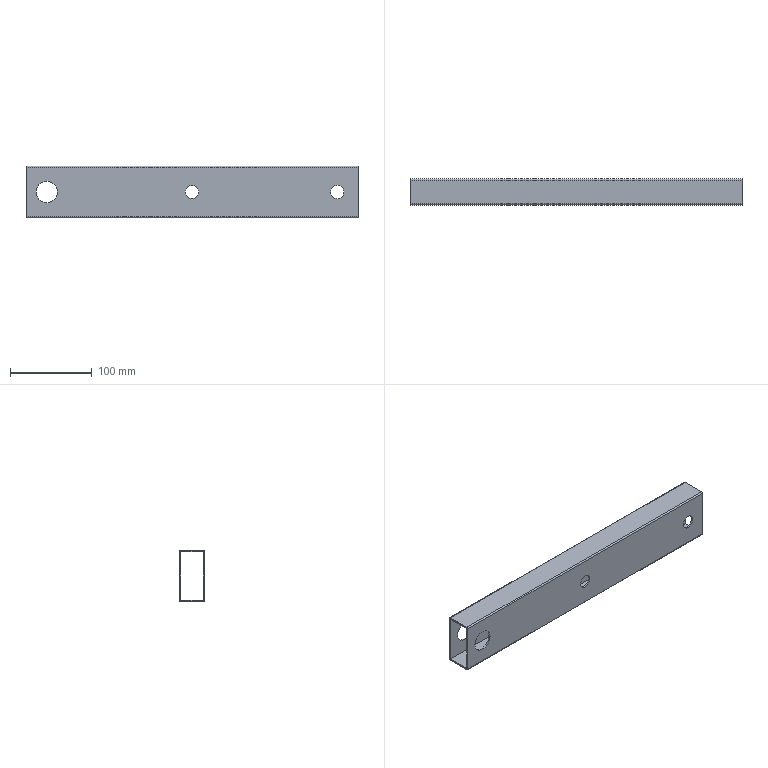Part | NX | features BREP 1 | 1 solid | 26 faces | box 406.4 x 31.75 x 63.5 mm | volume 142348 mm3 | cylinder 16 | plane 10 | commonest cylinder face diameters 16.256 x8 3.175 x4 26.162 x4
STEP:
#1=CARTESIAN_POINT('',(-203.2,15.875,-30.163));
#2=VERTEX_POINT('',#1);
#3=CARTESIAN_POINT('',(-203.2,15.875,30.163));
#4=VERTEX_POINT('',#3);
#5=CARTESIAN_POINT('',(-203.2,15.875,-30.163));
#6=DIRECTION('',(0.,0.,1.));
#7=VECTOR('',#6,1000.);
#8=LINE('',#5,#7);
#9=EDGE_CURVE('',#2,#4,#8,.T.);
#10=ORIENTED_EDGE('',*,*,#9,.F.);
#11=CARTESIAN_POINT('',(-203.2,14.287,-31.75));
#12=VERTEX_POINT('',#11);
#13=CARTESIAN_POINT('',(-203.2,14.287,-30.163));
#14=DIRECTION('',(-1.,0.,0.));
#15=DIRECTION('',(0.,1.,0.));
#16=AXIS2_PLACEMENT_3D('',#13,#14,#15);
#17=CIRCLE('',#16,1.587);
#18=EDGE_CURVE('',#2,#12,#17,.T.);
#19=ORIENTED_EDGE('',*,*,#18,.T.);
#20=CARTESIAN_POINT('',(-203.2,-14.287,-31.75));
#21=VERTEX_POINT('',#20);
#22=CARTESIAN_POINT('',(-203.2,-14.287,-31.75));
#23=DIRECTION('',(0.,1.,0.));
#24=VECTOR('',#23,1000.);
#25=LINE('',#22,#24);
#26=EDGE_CURVE('',#21,#12,#25,.T.);
#27=ORIENTED_EDGE('',*,*,#26,.F.);
#28=CARTESIAN_POINT('',(-203.2,-15.875,-30.163));
#29=VERTEX_POINT('',#28);
#30=CARTESIAN_POINT('',(-203.2,-14.287,-30.163));
#31=DIRECTION('',(-1.,0.,0.));
#32=DIRECTION('',(0.,0.,-1.));
#33=AXIS2_PLACEMENT_3D('',#30,#31,#32);
#34=CIRCLE('',#33,1.587);
#35=EDGE_CURVE('',#21,#29,#34,.T.);
#36=ORIENTED_EDGE('',*,*,#35,.T.);
#37=CARTESIAN_POINT('',(-203.2,-15.875,30.163));
#38=VERTEX_POINT('',#37);
#39=CARTESIAN_POINT('',(-203.2,-15.875,30.163));
#40=DIRECTION('',(0.,0.,-1.));
#41=VECTOR('',#40,1000.);
#42=LINE('',#39,#41);
#43=EDGE_CURVE('',#38,#29,#42,.T.);
#44=ORIENTED_EDGE('',*,*,#43,.F.);
#45=CARTESIAN_POINT('',(-203.2,-14.287,31.75));
#46=VERTEX_POINT('',#45);
#47=CARTESIAN_POINT('',(-203.2,-14.287,30.163));
#48=DIRECTION('',(-1.,0.,0.));
#49=DIRECTION('',(0.,-1.,0.));
#50=AXIS2_PLACEMENT_3D('',#47,#48,#49);
#51=CIRCLE('',#50,1.587);
#52=EDGE_CURVE('',#38,#46,#51,.T.);
#53=ORIENTED_EDGE('',*,*,#52,.T.);
#54=CARTESIAN_POINT('',(-203.2,14.287,31.75));
#55=VERTEX_POINT('',#54);
#56=CARTESIAN_POINT('',(-203.2,14.287,31.75));
#57=DIRECTION('',(0.,-1.,0.));
#58=VECTOR('',#57,1000.);
#59=LINE('',#56,#58);
#60=EDGE_CURVE('',#55,#46,#59,.T.);
#61=ORIENTED_EDGE('',*,*,#60,.F.);
#62=CARTESIAN_POINT('',(-203.2,14.287,30.163));
#63=DIRECTION('',(-1.,0.,0.));
#64=DIRECTION('',(0.,0.,1.));
#65=AXIS2_PLACEMENT_3D('',#62,#63,#64);
#66=CIRCLE('',#65,1.587);
#67=EDGE_CURVE('',#55,#4,#66,.T.);
#68=ORIENTED_EDGE('',*,*,#67,.T.);
#69=EDGE_LOOP('',(#10,#19,#27,#36,#44,#53,#61,#68));
#70=FACE_BOUND('',#69,.T.);
#71=CARTESIAN_POINT('',(-203.2,13.894,29.769));
#72=VERTEX_POINT('',#71);
#73=CARTESIAN_POINT('',(-203.2,13.894,-29.769));
#74=VERTEX_POINT('',#73);
#75=CARTESIAN_POINT('',(-203.2,13.894,29.769));
#76=DIRECTION('',(0.,0.,-1.));
#77=VECTOR('',#76,1000.);
#78=LINE('',#75,#77);
#79=EDGE_CURVE('',#72,#74,#78,.T.);
#80=ORIENTED_EDGE('',*,*,#79,.F.);
#81=CARTESIAN_POINT('',(-203.2,-13.894,29.769));
#82=VERTEX_POINT('',#81);
#83=CARTESIAN_POINT('',(-203.2,-13.894,29.769));
#84=DIRECTION('',(0.,1.,0.));
#85=VECTOR('',#84,1000.);
#86=LINE('',#83,#85);
#87=EDGE_CURVE('',#82,#72,#86,.T.);
#88=ORIENTED_EDGE('',*,*,#87,.F.);
#89=CARTESIAN_POINT('',(-203.2,-13.894,-29.769));
#90=VERTEX_POINT('',#89);
#91=CARTESIAN_POINT('',(-203.2,-13.894,-29.769));
#92=DIRECTION('',(0.,0.,1.));
#93=VECTOR('',#92,1000.);
#94=LINE('',#91,#93);
#95=EDGE_CURVE('',#90,#82,#94,.T.);
#96=ORIENTED_EDGE('',*,*,#95,.F.);
#97=CARTESIAN_POINT('',(-203.2,13.894,-29.769));
#98=DIRECTION('',(0.,-1.,0.));
#99=VECTOR('',#98,1000.);
#100=LINE('',#97,#99);
#101=EDGE_CURVE('',#74,#90,#100,.T.);
#102=ORIENTED_EDGE('',*,*,#101,.F.);
#103=EDGE_LOOP('',(#80,#88,#96,#102));
#104=FACE_BOUND('',#103,.T.);
#105=CARTESIAN_POINT('',(-203.2,0.,0.));
#106=DIRECTION('',(1.,0.,0.));
#107=DIRECTION('',(0.,1.,0.));
#108=AXIS2_PLACEMENT_3D('',#105,#106,#107);
#109=PLANE('',#108);
#110=ADVANCED_FACE('',(#70,#104),#109,.F.);
#111=CARTESIAN_POINT('',(203.2,-13.894,-29.769));
#112=VERTEX_POINT('',#111);
#113=CARTESIAN_POINT('',(-203.2,-13.894,-29.769));
#114=DIRECTION('',(1.,0.,0.));
#115=VECTOR('',#114,1000.);
#116=LINE('',#113,#115);
#117=EDGE_CURVE('',#90,#112,#116,.T.);
#118=ORIENTED_EDGE('',*,*,#117,.T.);
#119=CARTESIAN_POINT('',(203.2,13.894,-29.769));
#120=VERTEX_POINT('',#119);
#121=CARTESIAN_POINT('',(203.2,13.894,-29.769));
#122=DIRECTION('',(0.,-1.,0.));
#123=VECTOR('',#122,1000.);
#124=LINE('',#121,#123);
#125=EDGE_CURVE('',#120,#112,#124,.T.);
#126=ORIENTED_EDGE('',*,*,#125,.F.);
#127=CARTESIAN_POINT('',(-203.2,13.894,-29.769));
#128=DIRECTION('',(1.,0.,0.));
#129=VECTOR('',#128,1000.);
#130=LINE('',#127,#129);
#131=EDGE_CURVE('',#74,#120,#130,.T.);
#132=ORIENTED_EDGE('',*,*,#131,.F.);
#133=ORIENTED_EDGE('',*,*,#101,.T.);
#134=EDGE_LOOP('',(#118,#126,#132,#133));
#135=FACE_BOUND('',#134,.T.);
#136=CARTESIAN_POINT('',(-203.2,13.894,-29.769));
#137=DIRECTION('',(0.,0.,1.));
#138=DIRECTION('',(1.,0.,0.));
#139=AXIS2_PLACEMENT_3D('',#136,#137,#138);
#140=PLANE('',#139);
#141=ADVANCED_FACE('',(#135),#140,.T.);
#142=ORIENTED_EDGE('',*,*,#131,.T.);
#143=CARTESIAN_POINT('',(203.2,13.894,29.769));
#144=VERTEX_POINT('',#143);
#145=CARTESIAN_POINT('',(203.2,13.894,29.769));
#146=DIRECTION('',(0.,0.,-1.));
#147=VECTOR('',#146,1000.);
#148=LINE('',#145,#147);
#149=EDGE_CURVE('',#144,#120,#148,.T.);
#150=ORIENTED_EDGE('',*,*,#149,.F.);
#151=CARTESIAN_POINT('',(-203.2,13.894,29.769));
#152=DIRECTION('',(1.,0.,0.));
#153=VECTOR('',#152,1000.);
#154=LINE('',#151,#153);
#155=EDGE_CURVE('',#72,#144,#154,.T.);
#156=ORIENTED_EDGE('',*,*,#155,.F.);
#157=ORIENTED_EDGE('',*,*,#79,.T.);
#158=EDGE_LOOP('',(#142,#150,#156,#157));
#159=FACE_BOUND('',#158,.T.);
#160=CARTESIAN_POINT('',(-190.881,13.894,0.));
#161=VERTEX_POINT('',#160);
#162=CARTESIAN_POINT('',(-164.719,13.894,0.));
#163=VERTEX_POINT('',#162);
#164=CARTESIAN_POINT('',(-177.8,13.894,0.));
#165=DIRECTION('',(0.,-1.,0.));
#166=DIRECTION('',(-1.,0.,0.));
#167=AXIS2_PLACEMENT_3D('',#164,#165,#166);
#168=CIRCLE('',#167,13.081);
#169=EDGE_CURVE('',#161,#163,#168,.T.);
#170=ORIENTED_EDGE('',*,*,#169,.F.);
#171=CARTESIAN_POINT('',(-177.8,13.894,0.));
#172=DIRECTION('',(0.,-1.,0.));
#173=DIRECTION('',(1.,0.,0.));
#174=AXIS2_PLACEMENT_3D('',#171,#172,#173);
#175=CIRCLE('',#174,13.081);
#176=EDGE_CURVE('',#163,#161,#175,.T.);
#177=ORIENTED_EDGE('',*,*,#176,.F.);
#178=EDGE_LOOP('',(#170,#177));
#179=FACE_BOUND('',#178,.T.);
#180=CARTESIAN_POINT('',(169.672,13.894,0.));
#181=VERTEX_POINT('',#180);
#182=CARTESIAN_POINT('',(185.928,13.894,0.));
#183=VERTEX_POINT('',#182);
#184=CARTESIAN_POINT('',(177.8,13.894,0.));
#185=DIRECTION('',(0.,-1.,0.));
#186=DIRECTION('',(-1.,0.,0.));
#187=AXIS2_PLACEMENT_3D('',#184,#185,#186);
#188=CIRCLE('',#187,8.128);
#189=EDGE_CURVE('',#181,#183,#188,.T.);
#190=ORIENTED_EDGE('',*,*,#189,.F.);
#191=CARTESIAN_POINT('',(177.8,13.894,0.));
#192=DIRECTION('',(0.,-1.,0.));
#193=DIRECTION('',(1.,0.,0.));
#194=AXIS2_PLACEMENT_3D('',#191,#192,#193);
#195=CIRCLE('',#194,8.128);
#196=EDGE_CURVE('',#183,#181,#195,.T.);
#197=ORIENTED_EDGE('',*,*,#196,.F.);
#198=EDGE_LOOP('',(#190,#197));
#199=FACE_BOUND('',#198,.T.);
#200=CARTESIAN_POINT('',(-8.128,13.894,0.));
#201=VERTEX_POINT('',#200);
#202=CARTESIAN_POINT('',(8.128,13.894,0.));
#203=VERTEX_POINT('',#202);
#204=CARTESIAN_POINT('',(0.,13.894,0.));
#205=DIRECTION('',(0.,-1.,0.));
#206=DIRECTION('',(-1.,0.,0.));
#207=AXIS2_PLACEMENT_3D('',#204,#205,#206);
#208=CIRCLE('',#207,8.128);
#209=EDGE_CURVE('',#201,#203,#208,.T.);
#210=ORIENTED_EDGE('',*,*,#209,.F.);
#211=CARTESIAN_POINT('',(0.,13.894,0.));
#212=DIRECTION('',(0.,-1.,0.));
#213=DIRECTION('',(1.,0.,0.));
#214=AXIS2_PLACEMENT_3D('',#211,#212,#213);
#215=CIRCLE('',#214,8.128);
#216=EDGE_CURVE('',#203,#201,#215,.T.);
#217=ORIENTED_EDGE('',*,*,#216,.F.);
#218=EDGE_LOOP('',(#210,#217));
#219=FACE_BOUND('',#218,.T.);
#220=CARTESIAN_POINT('',(-203.2,13.894,29.769));
#221=DIRECTION('',(0.,-1.,0.));
#222=DIRECTION('',(0.,0.,-1.));
#223=AXIS2_PLACEMENT_3D('',#220,#221,#222);
#224=PLANE('',#223);
#225=ADVANCED_FACE('',(#159,#179,#199,#219),#224,.T.);
#226=ORIENTED_EDGE('',*,*,#155,.T.);
#227=CARTESIAN_POINT('',(203.2,-13.894,29.769));
#228=VERTEX_POINT('',#227);
#229=CARTESIAN_POINT('',(203.2,-13.894,29.769));
#230=DIRECTION('',(0.,1.,0.));
#231=VECTOR('',#230,1000.);
#232=LINE('',#229,#231);
#233=EDGE_CURVE('',#228,#144,#232,.T.);
#234=ORIENTED_EDGE('',*,*,#233,.F.);
#235=CARTESIAN_POINT('',(-203.2,-13.894,29.769));
#236=DIRECTION('',(1.,0.,0.));
#237=VECTOR('',#236,1000.);
#238=LINE('',#235,#237);
#239=EDGE_CURVE('',#82,#228,#238,.T.);
#240=ORIENTED_EDGE('',*,*,#239,.F.);
#241=ORIENTED_EDGE('',*,*,#87,.T.);
#242=EDGE_LOOP('',(#226,#234,#240,#241));
#243=FACE_BOUND('',#242,.T.);
#244=CARTESIAN_POINT('',(-203.2,-13.894,29.769));
#245=DIRECTION('',(0.,0.,-1.));
#246=DIRECTION('',(0.,-1.,0.));
#247=AXIS2_PLACEMENT_3D('',#244,#245,#246);
#248=PLANE('',#247);
#249=ADVANCED_FACE('',(#243),#248,.T.);
#250=ORIENTED_EDGE('',*,*,#239,.T.);
#251=CARTESIAN_POINT('',(203.2,-13.894,-29.769));
#252=DIRECTION('',(0.,0.,1.));
#253=VECTOR('',#252,1000.);
#254=LINE('',#251,#253);
#255=EDGE_CURVE('',#112,#228,#254,.T.);
#256=ORIENTED_EDGE('',*,*,#255,.F.);
#257=ORIENTED_EDGE('',*,*,#117,.F.);
#258=ORIENTED_EDGE('',*,*,#95,.T.);
#259=EDGE_LOOP('',(#250,#256,#257,#258));
#260=FACE_BOUND('',#259,.T.);
#261=CARTESIAN_POINT('',(-190.881,-13.894,0.));
#262=VERTEX_POINT('',#261);
#263=CARTESIAN_POINT('',(-164.719,-13.894,0.));
#264=VERTEX_POINT('',#263);
#265=CARTESIAN_POINT('',(-177.8,-13.894,0.));
#266=DIRECTION('',(0.,-1.,0.));
#267=DIRECTION('',(-1.,0.,0.));
#268=AXIS2_PLACEMENT_3D('',#265,#266,#267);
#269=CIRCLE('',#268,13.081);
#270=EDGE_CURVE('',#262,#264,#269,.T.);
#271=ORIENTED_EDGE('',*,*,#270,.T.);
#272=CARTESIAN_POINT('',(-177.8,-13.894,0.));
#273=DIRECTION('',(0.,-1.,0.));
#274=DIRECTION('',(1.,0.,0.));
#275=AXIS2_PLACEMENT_3D('',#272,#273,#274);
#276=CIRCLE('',#275,13.081);
#277=EDGE_CURVE('',#264,#262,#276,.T.);
#278=ORIENTED_EDGE('',*,*,#277,.T.);
#279=EDGE_LOOP('',(#271,#278));
#280=FACE_BOUND('',#279,.T.);
#281=CARTESIAN_POINT('',(169.672,-13.894,0.));
#282=VERTEX_POINT('',#281);
#283=CARTESIAN_POINT('',(185.928,-13.894,0.));
#284=VERTEX_POINT('',#283);
#285=CARTESIAN_POINT('',(177.8,-13.894,0.));
#286=DIRECTION('',(0.,-1.,0.));
#287=DIRECTION('',(-1.,0.,0.));
#288=AXIS2_PLACEMENT_3D('',#285,#286,#287);
#289=CIRCLE('',#288,8.128);
#290=EDGE_CURVE('',#282,#284,#289,.T.);
#291=ORIENTED_EDGE('',*,*,#290,.T.);
#292=CARTESIAN_POINT('',(177.8,-13.894,0.));
#293=DIRECTION('',(0.,-1.,0.));
#294=DIRECTION('',(1.,0.,0.));
#295=AXIS2_PLACEMENT_3D('',#292,#293,#294);
#296=CIRCLE('',#295,8.128);
#297=EDGE_CURVE('',#284,#282,#296,.T.);
#298=ORIENTED_EDGE('',*,*,#297,.T.);
#299=EDGE_LOOP('',(#291,#298));
#300=FACE_BOUND('',#299,.T.);
#301=CARTESIAN_POINT('',(-8.128,-13.894,0.));
#302=VERTEX_POINT('',#301);
#303=CARTESIAN_POINT('',(8.128,-13.894,0.));
#304=VERTEX_POINT('',#303);
#305=CARTESIAN_POINT('',(0.,-13.894,0.));
#306=DIRECTION('',(0.,-1.,0.));
#307=DIRECTION('',(-1.,0.,0.));
#308=AXIS2_PLACEMENT_3D('',#305,#306,#307);
#309=CIRCLE('',#308,8.128);
#310=EDGE_CURVE('',#302,#304,#309,.T.);
#311=ORIENTED_EDGE('',*,*,#310,.T.);
#312=CARTESIAN_POINT('',(0.,-13.894,0.));
#313=DIRECTION('',(0.,-1.,0.));
#314=DIRECTION('',(1.,0.,0.));
#315=AXIS2_PLACEMENT_3D('',#312,#313,#314);
#316=CIRCLE('',#315,8.128);
#317=EDGE_CURVE('',#304,#302,#316,.T.);
#318=ORIENTED_EDGE('',*,*,#317,.T.);
#319=EDGE_LOOP('',(#311,#318));
#320=FACE_BOUND('',#319,.T.);
#321=CARTESIAN_POINT('',(-203.2,-13.894,-29.769));
#322=DIRECTION('',(0.,1.,0.));
#323=DIRECTION('',(1.,0.,0.));
#324=AXIS2_PLACEMENT_3D('',#321,#322,#323);
#325=PLANE('',#324);
#326=ADVANCED_FACE('',(#260,#280,#300,#320),#325,.T.);
#327=CARTESIAN_POINT('',(203.2,14.287,31.75));
#328=VERTEX_POINT('',#327);
#329=CARTESIAN_POINT('',(203.2,-14.287,31.75));
#330=VERTEX_POINT('',#329);
#331=CARTESIAN_POINT('',(203.2,14.287,31.75));
#332=DIRECTION('',(0.,-1.,0.));
#333=VECTOR('',#332,1000.);
#334=LINE('',#331,#333);
#335=EDGE_CURVE('',#328,#330,#334,.T.);
#336=ORIENTED_EDGE('',*,*,#335,.T.);
#337=CARTESIAN_POINT('',(203.2,-15.875,30.163));
#338=VERTEX_POINT('',#337);
#339=CARTESIAN_POINT('',(203.2,-14.287,30.163));
#340=DIRECTION('',(1.,0.,0.));
#341=DIRECTION('',(0.,0.,1.));
#342=AXIS2_PLACEMENT_3D('',#339,#340,#341);
#343=CIRCLE('',#342,1.587);
#344=EDGE_CURVE('',#330,#338,#343,.T.);
#345=ORIENTED_EDGE('',*,*,#344,.T.);
#346=CARTESIAN_POINT('',(203.2,-15.875,-30.163));
#347=VERTEX_POINT('',#346);
#348=CARTESIAN_POINT('',(203.2,-15.875,30.163));
#349=DIRECTION('',(0.,0.,-1.));
#350=VECTOR('',#349,1000.);
#351=LINE('',#348,#350);
#352=EDGE_CURVE('',#338,#347,#351,.T.);
#353=ORIENTED_EDGE('',*,*,#352,.T.);
#354=CARTESIAN_POINT('',(203.2,-14.287,-31.75));
#355=VERTEX_POINT('',#354);
#356=CARTESIAN_POINT('',(203.2,-14.287,-30.163));
#357=DIRECTION('',(1.,0.,0.));
#358=DIRECTION('',(0.,-1.,0.));
#359=AXIS2_PLACEMENT_3D('',#356,#357,#358);
#360=CIRCLE('',#359,1.587);
#361=EDGE_CURVE('',#347,#355,#360,.T.);
#362=ORIENTED_EDGE('',*,*,#361,.T.);
#363=CARTESIAN_POINT('',(203.2,14.287,-31.75));
#364=VERTEX_POINT('',#363);
#365=CARTESIAN_POINT('',(203.2,-14.287,-31.75));
#366=DIRECTION('',(0.,1.,0.));
#367=VECTOR('',#366,1000.);
#368=LINE('',#365,#367);
#369=EDGE_CURVE('',#355,#364,#368,.T.);
#370=ORIENTED_EDGE('',*,*,#369,.T.);
#371=CARTESIAN_POINT('',(203.2,15.875,-30.163));
#372=VERTEX_POINT('',#371);
#373=CARTESIAN_POINT('',(203.2,14.287,-30.163));
#374=DIRECTION('',(1.,0.,0.));
#375=DIRECTION('',(0.,0.,-1.));
#376=AXIS2_PLACEMENT_3D('',#373,#374,#375);
#377=CIRCLE('',#376,1.587);
#378=EDGE_CURVE('',#364,#372,#377,.T.);
#379=ORIENTED_EDGE('',*,*,#378,.T.);
#380=CARTESIAN_POINT('',(203.2,15.875,30.163));
#381=VERTEX_POINT('',#380);
#382=CARTESIAN_POINT('',(203.2,15.875,-30.163));
#383=DIRECTION('',(0.,0.,1.));
#384=VECTOR('',#383,1000.);
#385=LINE('',#382,#384);
#386=EDGE_CURVE('',#372,#381,#385,.T.);
#387=ORIENTED_EDGE('',*,*,#386,.T.);
#388=CARTESIAN_POINT('',(203.2,14.287,30.163));
#389=DIRECTION('',(1.,0.,0.));
#390=DIRECTION('',(0.,1.,0.));
#391=AXIS2_PLACEMENT_3D('',#388,#389,#390);
#392=CIRCLE('',#391,1.587);
#393=EDGE_CURVE('',#381,#328,#392,.T.);
#394=ORIENTED_EDGE('',*,*,#393,.T.);
#395=EDGE_LOOP('',(#336,#345,#353,#362,#370,#379,#387,#394));
#396=FACE_BOUND('',#395,.T.);
#397=ORIENTED_EDGE('',*,*,#255,.T.);
#398=ORIENTED_EDGE('',*,*,#233,.T.);
#399=ORIENTED_EDGE('',*,*,#149,.T.);
#400=ORIENTED_EDGE('',*,*,#125,.T.);
#401=EDGE_LOOP('',(#397,#398,#399,#400));
#402=FACE_BOUND('',#401,.T.);
#403=CARTESIAN_POINT('',(203.2,0.,0.));
#404=DIRECTION('',(1.,0.,0.));
#405=DIRECTION('',(0.,1.,0.));
#406=AXIS2_PLACEMENT_3D('',#403,#404,#405);
#407=PLANE('',#406);
#408=ADVANCED_FACE('',(#396,#402),#407,.T.);
#409=ORIENTED_EDGE('',*,*,#393,.F.);
#410=CARTESIAN_POINT('',(203.2,15.875,30.163));
#411=DIRECTION('',(-1.,0.,0.));
#412=VECTOR('',#411,1000.);
#413=LINE('',#410,#412);
#414=EDGE_CURVE('',#381,#4,#413,.T.);
#415=ORIENTED_EDGE('',*,*,#414,.T.);
#416=ORIENTED_EDGE('',*,*,#67,.F.);
#417=CARTESIAN_POINT('',(203.2,14.287,31.75));
#418=DIRECTION('',(-1.,0.,0.));
#419=VECTOR('',#418,1000.);
#420=LINE('',#417,#419);
#421=EDGE_CURVE('',#328,#55,#420,.T.);
#422=ORIENTED_EDGE('',*,*,#421,.F.);
#423=EDGE_LOOP('',(#409,#415,#416,#422));
#424=FACE_BOUND('',#423,.T.);
#425=CARTESIAN_POINT('',(203.846,14.287,30.163));
#426=DIRECTION('',(-1.,0.,0.));
#427=DIRECTION('',(0.,0.,1.));
#428=AXIS2_PLACEMENT_3D('',#425,#426,#427);
#429=CYLINDRICAL_SURFACE('',#428,1.587);
#430=ADVANCED_FACE('',(#424),#429,.T.);
#431=ORIENTED_EDGE('',*,*,#60,.T.);
#432=CARTESIAN_POINT('',(203.2,-14.287,31.75));
#433=DIRECTION('',(-1.,0.,0.));
#434=VECTOR('',#433,1000.);
#435=LINE('',#432,#434);
#436=EDGE_CURVE('',#330,#46,#435,.T.);
#437=ORIENTED_EDGE('',*,*,#436,.F.);
#438=ORIENTED_EDGE('',*,*,#335,.F.);
#439=ORIENTED_EDGE('',*,*,#421,.T.);
#440=EDGE_LOOP('',(#431,#437,#438,#439));
#441=FACE_BOUND('',#440,.T.);
#442=CARTESIAN_POINT('',(-203.2,15.875,31.75));
#443=DIRECTION('',(0.,0.,1.));
#444=DIRECTION('',(1.,0.,0.));
#445=AXIS2_PLACEMENT_3D('',#442,#443,#444);
#446=PLANE('',#445);
#447=ADVANCED_FACE('',(#441),#446,.T.);
#448=ORIENTED_EDGE('',*,*,#344,.F.);
#449=ORIENTED_EDGE('',*,*,#436,.T.);
#450=ORIENTED_EDGE('',*,*,#52,.F.);
#451=CARTESIAN_POINT('',(203.2,-15.875,30.163));
#452=DIRECTION('',(-1.,0.,0.));
#453=VECTOR('',#452,1000.);
#454=LINE('',#451,#453);
#455=EDGE_CURVE('',#338,#38,#454,.T.);
#456=ORIENTED_EDGE('',*,*,#455,.F.);
#457=EDGE_LOOP('',(#448,#449,#450,#456));
#458=FACE_BOUND('',#457,.T.);
#459=CARTESIAN_POINT('',(203.846,-14.287,30.163));
#460=DIRECTION('',(-1.,0.,0.));
#461=DIRECTION('',(0.,-1.,0.));
#462=AXIS2_PLACEMENT_3D('',#459,#460,#461);
#463=CYLINDRICAL_SURFACE('',#462,1.587);
#464=ADVANCED_FACE('',(#458),#463,.T.);
#465=ORIENTED_EDGE('',*,*,#43,.T.);
#466=CARTESIAN_POINT('',(203.2,-15.875,-30.163));
#467=DIRECTION('',(-1.,0.,0.));
#468=VECTOR('',#467,1000.);
#469=LINE('',#466,#468);
#470=EDGE_CURVE('',#347,#29,#469,.T.);
#471=ORIENTED_EDGE('',*,*,#470,.F.);
#472=ORIENTED_EDGE('',*,*,#352,.F.);
#473=ORIENTED_EDGE('',*,*,#455,.T.);
#474=EDGE_LOOP('',(#465,#471,#472,#473));
#475=FACE_BOUND('',#474,.T.);
#476=CARTESIAN_POINT('',(-190.881,-15.875,0.));
#477=VERTEX_POINT('',#476);
#478=CARTESIAN_POINT('',(-164.719,-15.875,0.));
#479=VERTEX_POINT('',#478);
#480=CARTESIAN_POINT('',(-177.8,-15.875,0.));
#481=DIRECTION('',(0.,-1.,0.));
#482=DIRECTION('',(-1.,0.,0.));
#483=AXIS2_PLACEMENT_3D('',#480,#481,#482);
#484=CIRCLE('',#483,13.081);
#485=EDGE_CURVE('',#477,#479,#484,.T.);
#486=ORIENTED_EDGE('',*,*,#485,.F.);
#487=CARTESIAN_POINT('',(-177.8,-15.875,0.));
#488=DIRECTION('',(0.,-1.,0.));
#489=DIRECTION('',(1.,0.,0.));
#490=AXIS2_PLACEMENT_3D('',#487,#488,#489);
#491=CIRCLE('',#490,13.081);
#492=EDGE_CURVE('',#479,#477,#491,.T.);
#493=ORIENTED_EDGE('',*,*,#492,.F.);
#494=EDGE_LOOP('',(#486,#493));
#495=FACE_BOUND('',#494,.T.);
#496=CARTESIAN_POINT('',(169.672,-15.875,0.));
#497=VERTEX_POINT('',#496);
#498=CARTESIAN_POINT('',(185.928,-15.875,0.));
#499=VERTEX_POINT('',#498);
#500=CARTESIAN_POINT('',(177.8,-15.875,0.));
#501=DIRECTION('',(0.,-1.,0.));
#502=DIRECTION('',(-1.,0.,0.));
#503=AXIS2_PLACEMENT_3D('',#500,#501,#502);
#504=CIRCLE('',#503,8.128);
#505=EDGE_CURVE('',#497,#499,#504,.T.);
#506=ORIENTED_EDGE('',*,*,#505,.F.);
#507=CARTESIAN_POINT('',(177.8,-15.875,0.));
#508=DIRECTION('',(0.,-1.,0.));
#509=DIRECTION('',(1.,0.,0.));
#510=AXIS2_PLACEMENT_3D('',#507,#508,#509);
#511=CIRCLE('',#510,8.128);
#512=EDGE_CURVE('',#499,#497,#511,.T.);
#513=ORIENTED_EDGE('',*,*,#512,.F.);
#514=EDGE_LOOP('',(#506,#513));
#515=FACE_BOUND('',#514,.T.);
#516=CARTESIAN_POINT('',(-8.128,-15.875,0.));
#517=VERTEX_POINT('',#516);
#518=CARTESIAN_POINT('',(8.128,-15.875,0.));
#519=VERTEX_POINT('',#518);
#520=CARTESIAN_POINT('',(0.,-15.875,0.));
#521=DIRECTION('',(0.,-1.,0.));
#522=DIRECTION('',(-1.,0.,0.));
#523=AXIS2_PLACEMENT_3D('',#520,#521,#522);
#524=CIRCLE('',#523,8.128);
#525=EDGE_CURVE('',#517,#519,#524,.T.);
#526=ORIENTED_EDGE('',*,*,#525,.F.);
#527=CARTESIAN_POINT('',(0.,-15.875,0.));
#528=DIRECTION('',(0.,-1.,0.));
#529=DIRECTION('',(1.,0.,0.));
#530=AXIS2_PLACEMENT_3D('',#527,#528,#529);
#531=CIRCLE('',#530,8.128);
#532=EDGE_CURVE('',#519,#517,#531,.T.);
#533=ORIENTED_EDGE('',*,*,#532,.F.);
#534=EDGE_LOOP('',(#526,#533));
#535=FACE_BOUND('',#534,.T.);
#536=CARTESIAN_POINT('',(-203.2,-15.875,31.75));
#537=DIRECTION('',(0.,-1.,0.));
#538=DIRECTION('',(0.,0.,-1.));
#539=AXIS2_PLACEMENT_3D('',#536,#537,#538);
#540=PLANE('',#539);
#541=ADVANCED_FACE('',(#475,#495,#515,#535),#540,.T.);
#542=ORIENTED_EDGE('',*,*,#361,.F.);
#543=ORIENTED_EDGE('',*,*,#470,.T.);
#544=ORIENTED_EDGE('',*,*,#35,.F.);
#545=CARTESIAN_POINT('',(203.2,-14.287,-31.75));
#546=DIRECTION('',(-1.,0.,0.));
#547=VECTOR('',#546,1000.);
#548=LINE('',#545,#547);
#549=EDGE_CURVE('',#355,#21,#548,.T.);
#550=ORIENTED_EDGE('',*,*,#549,.F.);
#551=EDGE_LOOP('',(#542,#543,#544,#550));
#552=FACE_BOUND('',#551,.T.);
#553=CARTESIAN_POINT('',(203.846,-14.287,-30.163));
#554=DIRECTION('',(-1.,0.,0.));
#555=DIRECTION('',(0.,0.,-1.));
#556=AXIS2_PLACEMENT_3D('',#553,#554,#555);
#557=CYLINDRICAL_SURFACE('',#556,1.587);
#558=ADVANCED_FACE('',(#552),#557,.T.);
#559=ORIENTED_EDGE('',*,*,#369,.F.);
#560=ORIENTED_EDGE('',*,*,#549,.T.);
#561=ORIENTED_EDGE('',*,*,#26,.T.);
#562=CARTESIAN_POINT('',(203.2,14.287,-31.75));
#563=DIRECTION('',(-1.,0.,0.));
#564=VECTOR('',#563,1000.);
#565=LINE('',#562,#564);
#566=EDGE_CURVE('',#364,#12,#565,.T.);
#567=ORIENTED_EDGE('',*,*,#566,.F.);
#568=EDGE_LOOP('',(#559,#560,#561,#567));
#569=FACE_BOUND('',#568,.T.);
#570=CARTESIAN_POINT('',(-203.2,-15.875,-31.75));
#571=DIRECTION('',(0.,0.,-1.));
#572=DIRECTION('',(0.,-1.,0.));
#573=AXIS2_PLACEMENT_3D('',#570,#571,#572);
#574=PLANE('',#573);
#575=ADVANCED_FACE('',(#569),#574,.T.);
#576=ORIENTED_EDGE('',*,*,#378,.F.);
#577=ORIENTED_EDGE('',*,*,#566,.T.);
#578=ORIENTED_EDGE('',*,*,#18,.F.);
#579=CARTESIAN_POINT('',(203.2,15.875,-30.163));
#580=DIRECTION('',(-1.,0.,0.));
#581=VECTOR('',#580,1000.);
#582=LINE('',#579,#581);
#583=EDGE_CURVE('',#372,#2,#582,.T.);
#584=ORIENTED_EDGE('',*,*,#583,.F.);
#585=EDGE_LOOP('',(#576,#577,#578,#584));
#586=FACE_BOUND('',#585,.T.);
#587=CARTESIAN_POINT('',(203.846,14.287,-30.163));
#588=DIRECTION('',(-1.,0.,0.));
#589=DIRECTION('',(0.,1.,0.));
#590=AXIS2_PLACEMENT_3D('',#587,#588,#589);
#591=CYLINDRICAL_SURFACE('',#590,1.587);
#592=ADVANCED_FACE('',(#586),#591,.T.);
#593=ORIENTED_EDGE('',*,*,#386,.F.);
#594=ORIENTED_EDGE('',*,*,#583,.T.);
#595=ORIENTED_EDGE('',*,*,#9,.T.);
#596=ORIENTED_EDGE('',*,*,#414,.F.);
#597=EDGE_LOOP('',(#593,#594,#595,#596));
#598=FACE_BOUND('',#597,.T.);
#599=CARTESIAN_POINT('',(-190.881,15.875,0.));
#600=VERTEX_POINT('',#599);
#601=CARTESIAN_POINT('',(-164.719,15.875,0.));
#602=VERTEX_POINT('',#601);
#603=CARTESIAN_POINT('',(-177.8,15.875,0.));
#604=DIRECTION('',(0.,-1.,0.));
#605=DIRECTION('',(-1.,0.,0.));
#606=AXIS2_PLACEMENT_3D('',#603,#604,#605);
#607=CIRCLE('',#606,13.081);
#608=EDGE_CURVE('',#600,#602,#607,.T.);
#609=ORIENTED_EDGE('',*,*,#608,.T.);
#610=CARTESIAN_POINT('',(-177.8,15.875,0.));
#611=DIRECTION('',(0.,-1.,0.));
#612=DIRECTION('',(1.,0.,0.));
#613=AXIS2_PLACEMENT_3D('',#610,#611,#612);
#614=CIRCLE('',#613,13.081);
#615=EDGE_CURVE('',#602,#600,#614,.T.);
#616=ORIENTED_EDGE('',*,*,#615,.T.);
#617=EDGE_LOOP('',(#609,#616));
#618=FACE_BOUND('',#617,.T.);
#619=CARTESIAN_POINT('',(169.672,15.875,0.));
#620=VERTEX_POINT('',#619);
#621=CARTESIAN_POINT('',(185.928,15.875,0.));
#622=VERTEX_POINT('',#621);
#623=CARTESIAN_POINT('',(177.8,15.875,0.));
#624=DIRECTION('',(0.,-1.,0.));
#625=DIRECTION('',(-1.,0.,0.));
#626=AXIS2_PLACEMENT_3D('',#623,#624,#625);
#627=CIRCLE('',#626,8.128);
#628=EDGE_CURVE('',#620,#622,#627,.T.);
#629=ORIENTED_EDGE('',*,*,#628,.T.);
#630=CARTESIAN_POINT('',(177.8,15.875,0.));
#631=DIRECTION('',(0.,-1.,0.));
#632=DIRECTION('',(1.,0.,0.));
#633=AXIS2_PLACEMENT_3D('',#630,#631,#632);
#634=CIRCLE('',#633,8.128);
#635=EDGE_CURVE('',#622,#620,#634,.T.);
#636=ORIENTED_EDGE('',*,*,#635,.T.);
#637=EDGE_LOOP('',(#629,#636));
#638=FACE_BOUND('',#637,.T.);
#639=CARTESIAN_POINT('',(-8.128,15.875,0.));
#640=VERTEX_POINT('',#639);
#641=CARTESIAN_POINT('',(8.128,15.875,0.));
#642=VERTEX_POINT('',#641);
#643=CARTESIAN_POINT('',(0.,15.875,0.));
#644=DIRECTION('',(0.,-1.,0.));
#645=DIRECTION('',(-1.,0.,0.));
#646=AXIS2_PLACEMENT_3D('',#643,#644,#645);
#647=CIRCLE('',#646,8.128);
#648=EDGE_CURVE('',#640,#642,#647,.T.);
#649=ORIENTED_EDGE('',*,*,#648,.T.);
#650=CARTESIAN_POINT('',(0.,15.875,0.));
#651=DIRECTION('',(0.,-1.,0.));
#652=DIRECTION('',(1.,0.,0.));
#653=AXIS2_PLACEMENT_3D('',#650,#651,#652);
#654=CIRCLE('',#653,8.128);
#655=EDGE_CURVE('',#642,#640,#654,.T.);
#656=ORIENTED_EDGE('',*,*,#655,.T.);
#657=EDGE_LOOP('',(#649,#656));
#658=FACE_BOUND('',#657,.T.);
#659=CARTESIAN_POINT('',(-203.2,15.875,-31.75));
#660=DIRECTION('',(0.,1.,0.));
#661=DIRECTION('',(1.,0.,0.));
#662=AXIS2_PLACEMENT_3D('',#659,#660,#661);
#663=PLANE('',#662);
#664=ADVANCED_FACE('',(#598,#618,#638,#658),#663,.T.);
#665=CARTESIAN_POINT('',(-164.719,15.875,0.));
#666=DIRECTION('',(0.,-1.,0.));
#667=VECTOR('',#666,1000.);
#668=LINE('',#665,#667);
#669=EDGE_CURVE('',#163,#602,#668,.F.);
#670=ORIENTED_EDGE('',*,*,#669,.F.);
#671=ORIENTED_EDGE('',*,*,#176,.T.);
#672=CARTESIAN_POINT('',(-190.881,15.875,0.));
#673=DIRECTION('',(0.,-1.,0.));
#674=VECTOR('',#673,1000.);
#675=LINE('',#672,#674);
#676=EDGE_CURVE('',#161,#600,#675,.F.);
#677=ORIENTED_EDGE('',*,*,#676,.T.);
#678=ORIENTED_EDGE('',*,*,#615,.F.);
#679=EDGE_LOOP('',(#670,#671,#677,#678));
#680=FACE_BOUND('',#679,.T.);
#681=CARTESIAN_POINT('',(-177.8,15.875,0.));
#682=DIRECTION('',(0.,-1.,0.));
#683=DIRECTION('',(1.,0.,0.));
#684=AXIS2_PLACEMENT_3D('',#681,#682,#683);
#685=CYLINDRICAL_SURFACE('',#684,13.081);
#686=ADVANCED_FACE('',(#680),#685,.F.);
#687=CARTESIAN_POINT('',(-190.881,-13.894,0.));
#688=DIRECTION('',(0.,-1.,0.));
#689=VECTOR('',#688,1000.);
#690=LINE('',#687,#689);
#691=EDGE_CURVE('',#262,#477,#690,.T.);
#692=ORIENTED_EDGE('',*,*,#691,.F.);
#693=ORIENTED_EDGE('',*,*,#277,.F.);
#694=CARTESIAN_POINT('',(-164.719,-13.894,0.));
#695=DIRECTION('',(0.,-1.,0.));
#696=VECTOR('',#695,1000.);
#697=LINE('',#694,#696);
#698=EDGE_CURVE('',#264,#479,#697,.T.);
#699=ORIENTED_EDGE('',*,*,#698,.T.);
#700=ORIENTED_EDGE('',*,*,#492,.T.);
#701=EDGE_LOOP('',(#692,#693,#699,#700));
#702=FACE_BOUND('',#701,.T.);
#703=CARTESIAN_POINT('',(-177.8,15.875,0.));
#704=DIRECTION('',(0.,-1.,0.));
#705=DIRECTION('',(1.,0.,0.));
#706=AXIS2_PLACEMENT_3D('',#703,#704,#705);
#707=CYLINDRICAL_SURFACE('',#706,13.081);
#708=ADVANCED_FACE('',(#702),#707,.F.);
#709=ORIENTED_EDGE('',*,*,#676,.F.);
#710=ORIENTED_EDGE('',*,*,#169,.T.);
#711=ORIENTED_EDGE('',*,*,#669,.T.);
#712=ORIENTED_EDGE('',*,*,#608,.F.);
#713=EDGE_LOOP('',(#709,#710,#711,#712));
#714=FACE_BOUND('',#713,.T.);
#715=CARTESIAN_POINT('',(-177.8,15.875,0.));
#716=DIRECTION('',(0.,-1.,0.));
#717=DIRECTION('',(1.,0.,0.));
#718=AXIS2_PLACEMENT_3D('',#715,#716,#717);
#719=CYLINDRICAL_SURFACE('',#718,13.081);
#720=ADVANCED_FACE('',(#714),#719,.F.);
#721=ORIENTED_EDGE('',*,*,#698,.F.);
#722=ORIENTED_EDGE('',*,*,#270,.F.);
#723=ORIENTED_EDGE('',*,*,#691,.T.);
#724=ORIENTED_EDGE('',*,*,#485,.T.);
#725=EDGE_LOOP('',(#721,#722,#723,#724));
#726=FACE_BOUND('',#725,.T.);
#727=CARTESIAN_POINT('',(-177.8,15.875,0.));
#728=DIRECTION('',(0.,-1.,0.));
#729=DIRECTION('',(1.,0.,0.));
#730=AXIS2_PLACEMENT_3D('',#727,#728,#729);
#731=CYLINDRICAL_SURFACE('',#730,13.081);
#732=ADVANCED_FACE('',(#726),#731,.F.);
#733=CARTESIAN_POINT('',(185.928,15.875,0.));
#734=DIRECTION('',(0.,-1.,0.));
#735=VECTOR('',#734,1000.);
#736=LINE('',#733,#735);
#737=EDGE_CURVE('',#183,#622,#736,.F.);
#738=ORIENTED_EDGE('',*,*,#737,.F.);
#739=ORIENTED_EDGE('',*,*,#196,.T.);
#740=CARTESIAN_POINT('',(169.672,15.875,0.));
#741=DIRECTION('',(0.,-1.,0.));
#742=VECTOR('',#741,1000.);
#743=LINE('',#740,#742);
#744=EDGE_CURVE('',#181,#620,#743,.F.);
#745=ORIENTED_EDGE('',*,*,#744,.T.);
#746=ORIENTED_EDGE('',*,*,#635,.F.);
#747=EDGE_LOOP('',(#738,#739,#745,#746));
#748=FACE_BOUND('',#747,.T.);
#749=CARTESIAN_POINT('',(177.8,15.875,0.));
#750=DIRECTION('',(0.,-1.,0.));
#751=DIRECTION('',(1.,0.,0.));
#752=AXIS2_PLACEMENT_3D('',#749,#750,#751);
#753=CYLINDRICAL_SURFACE('',#752,8.128);
#754=ADVANCED_FACE('',(#748),#753,.F.);
#755=CARTESIAN_POINT('',(169.672,-13.894,0.));
#756=DIRECTION('',(0.,-1.,0.));
#757=VECTOR('',#756,1000.);
#758=LINE('',#755,#757);
#759=EDGE_CURVE('',#282,#497,#758,.T.);
#760=ORIENTED_EDGE('',*,*,#759,.F.);
#761=ORIENTED_EDGE('',*,*,#297,.F.);
#762=CARTESIAN_POINT('',(185.928,-13.894,0.));
#763=DIRECTION('',(0.,-1.,0.));
#764=VECTOR('',#763,1000.);
#765=LINE('',#762,#764);
#766=EDGE_CURVE('',#284,#499,#765,.T.);
#767=ORIENTED_EDGE('',*,*,#766,.T.);
#768=ORIENTED_EDGE('',*,*,#512,.T.);
#769=EDGE_LOOP('',(#760,#761,#767,#768));
#770=FACE_BOUND('',#769,.T.);
#771=CARTESIAN_POINT('',(177.8,15.875,0.));
#772=DIRECTION('',(0.,-1.,0.));
#773=DIRECTION('',(1.,0.,0.));
#774=AXIS2_PLACEMENT_3D('',#771,#772,#773);
#775=CYLINDRICAL_SURFACE('',#774,8.128);
#776=ADVANCED_FACE('',(#770),#775,.F.);
#777=ORIENTED_EDGE('',*,*,#744,.F.);
#778=ORIENTED_EDGE('',*,*,#189,.T.);
#779=ORIENTED_EDGE('',*,*,#737,.T.);
#780=ORIENTED_EDGE('',*,*,#628,.F.);
#781=EDGE_LOOP('',(#777,#778,#779,#780));
#782=FACE_BOUND('',#781,.T.);
#783=CARTESIAN_POINT('',(177.8,15.875,0.));
#784=DIRECTION('',(0.,-1.,0.));
#785=DIRECTION('',(1.,0.,0.));
#786=AXIS2_PLACEMENT_3D('',#783,#784,#785);
#787=CYLINDRICAL_SURFACE('',#786,8.128);
#788=ADVANCED_FACE('',(#782),#787,.F.);
#789=ORIENTED_EDGE('',*,*,#766,.F.);
#790=ORIENTED_EDGE('',*,*,#290,.F.);
#791=ORIENTED_EDGE('',*,*,#759,.T.);
#792=ORIENTED_EDGE('',*,*,#505,.T.);
#793=EDGE_LOOP('',(#789,#790,#791,#792));
#794=FACE_BOUND('',#793,.T.);
#795=CARTESIAN_POINT('',(177.8,15.875,0.));
#796=DIRECTION('',(0.,-1.,0.));
#797=DIRECTION('',(1.,0.,0.));
#798=AXIS2_PLACEMENT_3D('',#795,#796,#797);
#799=CYLINDRICAL_SURFACE('',#798,8.128);
#800=ADVANCED_FACE('',(#794),#799,.F.);
#801=CARTESIAN_POINT('',(8.128,15.875,0.));
#802=DIRECTION('',(0.,-1.,0.));
#803=VECTOR('',#802,1000.);
#804=LINE('',#801,#803);
#805=EDGE_CURVE('',#203,#642,#804,.F.);
#806=ORIENTED_EDGE('',*,*,#805,.F.);
#807=ORIENTED_EDGE('',*,*,#216,.T.);
#808=CARTESIAN_POINT('',(-8.128,15.875,0.));
#809=DIRECTION('',(0.,-1.,0.));
#810=VECTOR('',#809,1000.);
#811=LINE('',#808,#810);
#812=EDGE_CURVE('',#201,#640,#811,.F.);
#813=ORIENTED_EDGE('',*,*,#812,.T.);
#814=ORIENTED_EDGE('',*,*,#655,.F.);
#815=EDGE_LOOP('',(#806,#807,#813,#814));
#816=FACE_BOUND('',#815,.T.);
#817=CARTESIAN_POINT('',(0.,15.875,0.));
#818=DIRECTION('',(0.,-1.,0.));
#819=DIRECTION('',(1.,0.,0.));
#820=AXIS2_PLACEMENT_3D('',#817,#818,#819);
#821=CYLINDRICAL_SURFACE('',#820,8.128);
#822=ADVANCED_FACE('',(#816),#821,.F.);
#823=CARTESIAN_POINT('',(-8.128,-13.894,0.));
#824=DIRECTION('',(0.,-1.,0.));
#825=VECTOR('',#824,1000.);
#826=LINE('',#823,#825);
#827=EDGE_CURVE('',#302,#517,#826,.T.);
#828=ORIENTED_EDGE('',*,*,#827,.F.);
#829=ORIENTED_EDGE('',*,*,#317,.F.);
#830=CARTESIAN_POINT('',(8.128,-13.894,0.));
#831=DIRECTION('',(0.,-1.,0.));
#832=VECTOR('',#831,1000.);
#833=LINE('',#830,#832);
#834=EDGE_CURVE('',#304,#519,#833,.T.);
#835=ORIENTED_EDGE('',*,*,#834,.T.);
#836=ORIENTED_EDGE('',*,*,#532,.T.);
#837=EDGE_LOOP('',(#828,#829,#835,#836));
#838=FACE_BOUND('',#837,.T.);
#839=CARTESIAN_POINT('',(0.,15.875,0.));
#840=DIRECTION('',(0.,-1.,0.));
#841=DIRECTION('',(1.,0.,0.));
#842=AXIS2_PLACEMENT_3D('',#839,#840,#841);
#843=CYLINDRICAL_SURFACE('',#842,8.128);
#844=ADVANCED_FACE('',(#838),#843,.F.);
#845=ORIENTED_EDGE('',*,*,#812,.F.);
#846=ORIENTED_EDGE('',*,*,#209,.T.);
#847=ORIENTED_EDGE('',*,*,#805,.T.);
#848=ORIENTED_EDGE('',*,*,#648,.F.);
#849=EDGE_LOOP('',(#845,#846,#847,#848));
#850=FACE_BOUND('',#849,.T.);
#851=CARTESIAN_POINT('',(0.,15.875,0.));
#852=DIRECTION('',(0.,-1.,0.));
#853=DIRECTION('',(1.,0.,0.));
#854=AXIS2_PLACEMENT_3D('',#851,#852,#853);
#855=CYLINDRICAL_SURFACE('',#854,8.128);
#856=ADVANCED_FACE('',(#850),#855,.F.);
#857=ORIENTED_EDGE('',*,*,#834,.F.);
#858=ORIENTED_EDGE('',*,*,#310,.F.);
#859=ORIENTED_EDGE('',*,*,#827,.T.);
#860=ORIENTED_EDGE('',*,*,#525,.T.);
#861=EDGE_LOOP('',(#857,#858,#859,#860));
#862=FACE_BOUND('',#861,.T.);
#863=CARTESIAN_POINT('',(0.,15.875,0.));
#864=DIRECTION('',(0.,-1.,0.));
#865=DIRECTION('',(1.,0.,0.));
#866=AXIS2_PLACEMENT_3D('',#863,#864,#865);
#867=CYLINDRICAL_SURFACE('',#866,8.128);
#868=ADVANCED_FACE('',(#862),#867,.F.);
#869=CLOSED_SHELL('',(#110,#141,#225,#249,#326,#408,#430,#447,#464,#541,#558,#575,#592,#664,#686,#708,#720,#732,#754,#776,#788,#800,#822,#844,#856,#868));
#870=MANIFOLD_SOLID_BREP('',#869);
#871=(LENGTH_UNIT()NAMED_UNIT(*)SI_UNIT(.MILLI.,.METRE.));
#872=UNCERTAINTY_MEASURE_WITH_UNIT(LENGTH_MEASURE(0.00001),#871,'','');
#873=(NAMED_UNIT(*)PLANE_ANGLE_UNIT()SI_UNIT($,.RADIAN.));
#874=(NAMED_UNIT(*)SI_UNIT($,.STERADIAN.)SOLID_ANGLE_UNIT());
#875=(GEOMETRIC_REPRESENTATION_CONTEXT(3)GLOBAL_UNCERTAINTY_ASSIGNED_CONTEXT((#872))GLOBAL_UNIT_ASSIGNED_CONTEXT((#871,#873,#874))REPRESENTATION_CONTEXT('',''));
#876=ADVANCED_BREP_SHAPE_REPRESENTATION('',(#870),#875);